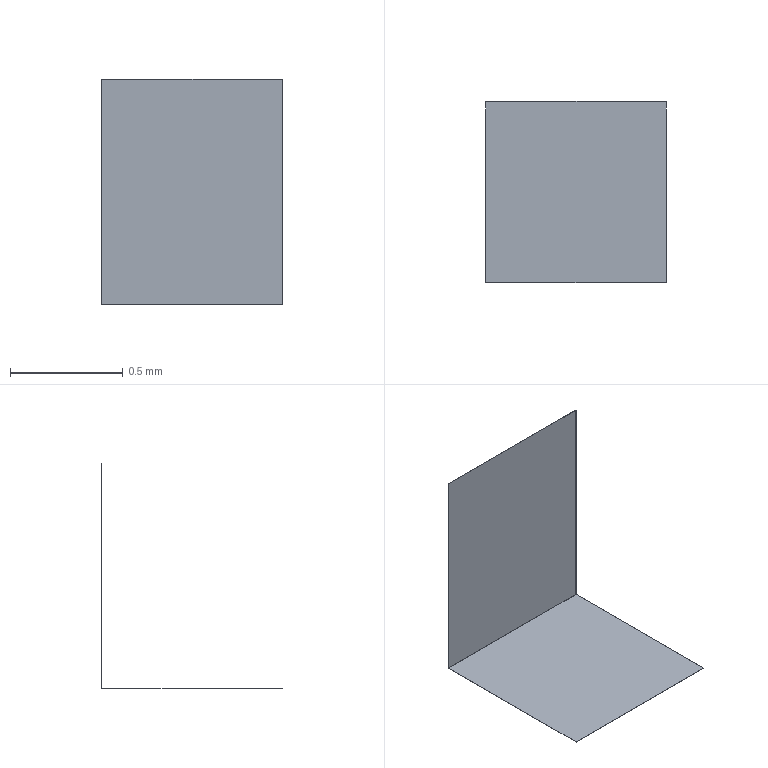Part | STEP file | RJ-USIO-V1_2-220411_9 | 1 solid | 14 faces | box 0.8 x 0.801 x 1 mm | volume 0.00144 mm3 | plane 14
STEP:
#1=CARTESIAN_POINT('',(0.,0.,0.));
#2=DIRECTION('',(0.,0.,1.));
#3=DIRECTION('',(1.,0.,0.));
#4=AXIS2_PLACEMENT_3D('',#1,#2,#3);
#5=CARTESIAN_POINT('',(24.9,60.501,1.));
#6=VERTEX_POINT('',#5);
#7=CARTESIAN_POINT('',(24.1,60.501,1.));
#8=VERTEX_POINT('',#7);
#9=CARTESIAN_POINT('',(24.9,60.501,1.));
#10=DIRECTION('',(-1.,-0.000000012,0.));
#11=VECTOR('',#10,1.);
#12=LINE('',#9,#11);
#13=CARTESIAN_POINT('',(24.1,60.501,0.));
#14=DIRECTION('',(0.000000012,-1.,0.));
#15=DIRECTION('',(0.,0.,1.));
#16=AXIS2_PLACEMENT_3D('',#13,#14,#15);
#17=PLANE('',#16);
#18=CARTESIAN_POINT('',(1.,-0.8));
#19=DIRECTION('',(0.,1.));
#20=VECTOR('',#19,1.);
#21=LINE('',#18,#20);
#22=(GEOMETRIC_REPRESENTATION_CONTEXT(2)PARAMETRIC_REPRESENTATION_CONTEXT()REPRESENTATION_CONTEXT('',''));
#23=DEFINITIONAL_REPRESENTATION('',(#21),#22);
#24=PCURVE('',#17,#23);
#25=CARTESIAN_POINT('',(24.1,60.5,1.));
#26=DIRECTION('',(0.,0.,-1.));
#27=DIRECTION('',(-1.,-0.000000012,0.));
#28=AXIS2_PLACEMENT_3D('',#25,#26,#27);
#29=PLANE('',#28);
#30=CARTESIAN_POINT('',(-0.8,0.001));
#31=DIRECTION('',(1.,0.));
#32=VECTOR('',#31,1.);
#33=LINE('',#30,#32);
#34=(GEOMETRIC_REPRESENTATION_CONTEXT(2)PARAMETRIC_REPRESENTATION_CONTEXT()REPRESENTATION_CONTEXT('',''));
#35=DEFINITIONAL_REPRESENTATION('',(#33),#34);
#36=PCURVE('',#29,#35);
#37=SURFACE_CURVE('',#12,(#24,#36),.PCURVE_S1.);
#38=EDGE_CURVE('',#6,#8,#37,.T.);
#39=ORIENTED_EDGE('',*,*,#38,.T.);
#40=CARTESIAN_POINT('',(24.1,60.501,0.001));
#41=VERTEX_POINT('',#40);
#42=CARTESIAN_POINT('',(24.1,60.501,1.));
#43=DIRECTION('',(0.,0.,-1.));
#44=VECTOR('',#43,1.);
#45=LINE('',#42,#44);
#46=CARTESIAN_POINT('',(1.,0.));
#47=DIRECTION('',(-1.,0.));
#48=VECTOR('',#47,1.);
#49=LINE('',#46,#48);
#50=(GEOMETRIC_REPRESENTATION_CONTEXT(2)PARAMETRIC_REPRESENTATION_CONTEXT()REPRESENTATION_CONTEXT('',''));
#51=DEFINITIONAL_REPRESENTATION('',(#49),#50);
#52=PCURVE('',#17,#51);
#53=CARTESIAN_POINT('',(24.1,60.5,0.));
#54=DIRECTION('',(1.,0.000000012,0.));
#55=DIRECTION('',(0.,0.,-1.));
#56=AXIS2_PLACEMENT_3D('',#53,#54,#55);
#57=PLANE('',#56);
#58=CARTESIAN_POINT('',(-1.,0.001));
#59=DIRECTION('',(1.,0.));
#60=VECTOR('',#59,1.);
#61=LINE('',#58,#60);
#62=(GEOMETRIC_REPRESENTATION_CONTEXT(2)PARAMETRIC_REPRESENTATION_CONTEXT()REPRESENTATION_CONTEXT('',''));
#63=DEFINITIONAL_REPRESENTATION('',(#61),#62);
#64=PCURVE('',#57,#63);
#65=SURFACE_CURVE('',#45,(#52,#64),.PCURVE_S1.);
#66=EDGE_CURVE('',#8,#41,#65,.T.);
#67=ORIENTED_EDGE('',*,*,#66,.T.);
#68=CARTESIAN_POINT('',(24.9,60.501,0.001));
#69=VERTEX_POINT('',#68);
#70=CARTESIAN_POINT('',(24.1,60.501,0.001));
#71=DIRECTION('',(1.,0.000000012,0.));
#72=VECTOR('',#71,1.);
#73=LINE('',#70,#72);
#74=CARTESIAN_POINT('',(0.001,0.));
#75=DIRECTION('',(0.,-1.));
#76=VECTOR('',#75,1.);
#77=LINE('',#74,#76);
#78=(GEOMETRIC_REPRESENTATION_CONTEXT(2)PARAMETRIC_REPRESENTATION_CONTEXT()REPRESENTATION_CONTEXT('',''));
#79=DEFINITIONAL_REPRESENTATION('',(#77),#78);
#80=PCURVE('',#17,#79);
#81=CARTESIAN_POINT('',(24.9,60.501,0.));
#82=DIRECTION('',(0.000000012,-1.,0.));
#83=DIRECTION('',(1.,0.000000012,0.));
#84=AXIS2_PLACEMENT_3D('',#81,#82,#83);
#85=PLANE('',#84);
#86=CARTESIAN_POINT('',(-0.8,0.001));
#87=DIRECTION('',(1.,0.));
#88=VECTOR('',#87,1.);
#89=LINE('',#86,#88);
#90=(GEOMETRIC_REPRESENTATION_CONTEXT(2)PARAMETRIC_REPRESENTATION_CONTEXT()REPRESENTATION_CONTEXT('',''));
#91=DEFINITIONAL_REPRESENTATION('',(#89),#90);
#92=PCURVE('',#85,#91);
#93=SURFACE_CURVE('',#73,(#80,#92),.PCURVE_S1.);
#94=EDGE_CURVE('',#41,#69,#93,.T.);
#95=ORIENTED_EDGE('',*,*,#94,.T.);
#96=CARTESIAN_POINT('',(24.9,60.501,0.001));
#97=DIRECTION('',(0.,0.,1.));
#98=VECTOR('',#97,1.);
#99=LINE('',#96,#98);
#100=CARTESIAN_POINT('',(0.001,-0.8));
#101=DIRECTION('',(1.,0.));
#102=VECTOR('',#101,1.);
#103=LINE('',#100,#102);
#104=(GEOMETRIC_REPRESENTATION_CONTEXT(2)PARAMETRIC_REPRESENTATION_CONTEXT()REPRESENTATION_CONTEXT('',''));
#105=DEFINITIONAL_REPRESENTATION('',(#103),#104);
#106=PCURVE('',#17,#105);
#107=CARTESIAN_POINT('',(24.9,60.5,1.));
#108=DIRECTION('',(-1.,-0.000000012,0.));
#109=DIRECTION('',(0.,0.,1.));
#110=AXIS2_PLACEMENT_3D('',#107,#108,#109);
#111=PLANE('',#110);
#112=CARTESIAN_POINT('',(-0.999,0.001));
#113=DIRECTION('',(1.,0.));
#114=VECTOR('',#113,1.);
#115=LINE('',#112,#114);
#116=(GEOMETRIC_REPRESENTATION_CONTEXT(2)PARAMETRIC_REPRESENTATION_CONTEXT()REPRESENTATION_CONTEXT('',''));
#117=DEFINITIONAL_REPRESENTATION('',(#115),#116);
#118=PCURVE('',#111,#117);
#119=SURFACE_CURVE('',#99,(#106,#118),.PCURVE_S1.);
#120=EDGE_CURVE('',#69,#6,#119,.T.);
#121=ORIENTED_EDGE('',*,*,#120,.T.);
#122=EDGE_LOOP('',(#39,#67,#95,#121));
#123=FACE_BOUND('',#122,.F.);
#124=ADVANCED_FACE('',(#123),#17,.F.);
#125=CARTESIAN_POINT('',(24.9,60.5,1.));
#126=VERTEX_POINT('',#125);
#127=CARTESIAN_POINT('',(24.1,60.5,1.));
#128=VERTEX_POINT('',#127);
#129=CARTESIAN_POINT('',(24.9,60.5,1.));
#130=DIRECTION('',(-1.,-0.000000012,0.));
#131=VECTOR('',#130,1.);
#132=LINE('',#129,#131);
#133=CARTESIAN_POINT('',(-0.8,0.));
#134=DIRECTION('',(1.,0.));
#135=VECTOR('',#134,1.);
#136=LINE('',#133,#135);
#137=(GEOMETRIC_REPRESENTATION_CONTEXT(2)PARAMETRIC_REPRESENTATION_CONTEXT()REPRESENTATION_CONTEXT('',''));
#138=DEFINITIONAL_REPRESENTATION('',(#136),#137);
#139=PCURVE('',#29,#138);
#140=CARTESIAN_POINT('',(24.1,60.5,0.));
#141=DIRECTION('',(0.000000012,-1.,0.));
#142=DIRECTION('',(0.,0.,1.));
#143=AXIS2_PLACEMENT_3D('',#140,#141,#142);
#144=PLANE('',#143);
#145=CARTESIAN_POINT('',(1.,-0.8));
#146=DIRECTION('',(0.,1.));
#147=VECTOR('',#146,1.);
#148=LINE('',#145,#147);
#149=(GEOMETRIC_REPRESENTATION_CONTEXT(2)PARAMETRIC_REPRESENTATION_CONTEXT()REPRESENTATION_CONTEXT('',''));
#150=DEFINITIONAL_REPRESENTATION('',(#148),#149);
#151=PCURVE('',#144,#150);
#152=SURFACE_CURVE('',#132,(#139,#151),.PCURVE_S1.);
#153=EDGE_CURVE('',#126,#128,#152,.T.);
#154=ORIENTED_EDGE('',*,*,#153,.T.);
#155=CARTESIAN_POINT('',(24.1,60.501,1.));
#156=DIRECTION('',(0.000000012,-1.,0.));
#157=VECTOR('',#156,1.);
#158=LINE('',#155,#157);
#159=CARTESIAN_POINT('',(0.,0.001));
#160=DIRECTION('',(0.,-1.));
#161=VECTOR('',#160,1.);
#162=LINE('',#159,#161);
#163=(GEOMETRIC_REPRESENTATION_CONTEXT(2)PARAMETRIC_REPRESENTATION_CONTEXT()REPRESENTATION_CONTEXT('',''));
#164=DEFINITIONAL_REPRESENTATION('',(#162),#163);
#165=PCURVE('',#29,#164);
#166=CARTESIAN_POINT('',(-1.,0.001));
#167=DIRECTION('',(0.,-1.));
#168=VECTOR('',#167,1.);
#169=LINE('',#166,#168);
#170=(GEOMETRIC_REPRESENTATION_CONTEXT(2)PARAMETRIC_REPRESENTATION_CONTEXT()REPRESENTATION_CONTEXT('',''));
#171=DEFINITIONAL_REPRESENTATION('',(#169),#170);
#172=PCURVE('',#57,#171);
#173=SURFACE_CURVE('',#158,(#165,#172),.PCURVE_S1.);
#174=EDGE_CURVE('',#8,#128,#173,.T.);
#175=ORIENTED_EDGE('',*,*,#174,.F.);
#176=ORIENTED_EDGE('',*,*,#38,.F.);
#177=CARTESIAN_POINT('',(24.9,60.501,1.));
#178=DIRECTION('',(0.000000012,-1.,0.));
#179=VECTOR('',#178,1.);
#180=LINE('',#177,#179);
#181=CARTESIAN_POINT('',(-0.8,0.001));
#182=DIRECTION('',(0.,-1.));
#183=VECTOR('',#182,1.);
#184=LINE('',#181,#183);
#185=(GEOMETRIC_REPRESENTATION_CONTEXT(2)PARAMETRIC_REPRESENTATION_CONTEXT()REPRESENTATION_CONTEXT('',''));
#186=DEFINITIONAL_REPRESENTATION('',(#184),#185);
#187=PCURVE('',#29,#186);
#188=CARTESIAN_POINT('',(0.,0.001));
#189=DIRECTION('',(0.,-1.));
#190=VECTOR('',#189,1.);
#191=LINE('',#188,#190);
#192=(GEOMETRIC_REPRESENTATION_CONTEXT(2)PARAMETRIC_REPRESENTATION_CONTEXT()REPRESENTATION_CONTEXT('',''));
#193=DEFINITIONAL_REPRESENTATION('',(#191),#192);
#194=PCURVE('',#111,#193);
#195=SURFACE_CURVE('',#180,(#187,#194),.PCURVE_S1.);
#196=EDGE_CURVE('',#6,#126,#195,.T.);
#197=ORIENTED_EDGE('',*,*,#196,.T.);
#198=EDGE_LOOP('',(#154,#175,#176,#197));
#199=FACE_BOUND('',#198,.F.);
#200=ADVANCED_FACE('',(#199),#29,.F.);
#201=CARTESIAN_POINT('',(24.1,60.5,0.001));
#202=VERTEX_POINT('',#201);
#203=CARTESIAN_POINT('',(24.1,60.5,1.));
#204=DIRECTION('',(0.,0.,-1.));
#205=VECTOR('',#204,1.);
#206=LINE('',#203,#205);
#207=CARTESIAN_POINT('',(1.,0.));
#208=DIRECTION('',(-1.,0.));
#209=VECTOR('',#208,1.);
#210=LINE('',#207,#209);
#211=(GEOMETRIC_REPRESENTATION_CONTEXT(2)PARAMETRIC_REPRESENTATION_CONTEXT()REPRESENTATION_CONTEXT('',''));
#212=DEFINITIONAL_REPRESENTATION('',(#210),#211);
#213=PCURVE('',#144,#212);
#214=CARTESIAN_POINT('',(-1.,0.));
#215=DIRECTION('',(1.,0.));
#216=VECTOR('',#215,1.);
#217=LINE('',#214,#216);
#218=(GEOMETRIC_REPRESENTATION_CONTEXT(2)PARAMETRIC_REPRESENTATION_CONTEXT()REPRESENTATION_CONTEXT('',''));
#219=DEFINITIONAL_REPRESENTATION('',(#217),#218);
#220=PCURVE('',#57,#219);
#221=SURFACE_CURVE('',#206,(#213,#220),.PCURVE_S1.);
#222=EDGE_CURVE('',#128,#202,#221,.T.);
#223=ORIENTED_EDGE('',*,*,#222,.F.);
#224=ORIENTED_EDGE('',*,*,#153,.F.);
#225=CARTESIAN_POINT('',(24.9,60.5,0.001));
#226=VERTEX_POINT('',#225);
#227=CARTESIAN_POINT('',(24.9,60.5,0.001));
#228=DIRECTION('',(0.,0.,1.));
#229=VECTOR('',#228,1.);
#230=LINE('',#227,#229);
#231=CARTESIAN_POINT('',(0.001,-0.8));
#232=DIRECTION('',(1.,0.));
#233=VECTOR('',#232,1.);
#234=LINE('',#231,#233);
#235=(GEOMETRIC_REPRESENTATION_CONTEXT(2)PARAMETRIC_REPRESENTATION_CONTEXT()REPRESENTATION_CONTEXT('',''));
#236=DEFINITIONAL_REPRESENTATION('',(#234),#235);
#237=PCURVE('',#144,#236);
#238=CARTESIAN_POINT('',(-0.999,0.));
#239=DIRECTION('',(1.,0.));
#240=VECTOR('',#239,1.);
#241=LINE('',#238,#240);
#242=(GEOMETRIC_REPRESENTATION_CONTEXT(2)PARAMETRIC_REPRESENTATION_CONTEXT()REPRESENTATION_CONTEXT('',''));
#243=DEFINITIONAL_REPRESENTATION('',(#241),#242);
#244=PCURVE('',#111,#243);
#245=SURFACE_CURVE('',#230,(#237,#244),.PCURVE_S1.);
#246=EDGE_CURVE('',#226,#126,#245,.T.);
#247=ORIENTED_EDGE('',*,*,#246,.F.);
#248=CARTESIAN_POINT('',(24.1,60.5,0.001));
#249=DIRECTION('',(1.,0.000000012,0.));
#250=VECTOR('',#249,1.);
#251=LINE('',#248,#250);
#252=CARTESIAN_POINT('',(0.001,0.));
#253=DIRECTION('',(0.,-1.));
#254=VECTOR('',#253,1.);
#255=LINE('',#252,#254);
#256=(GEOMETRIC_REPRESENTATION_CONTEXT(2)PARAMETRIC_REPRESENTATION_CONTEXT()REPRESENTATION_CONTEXT('',''));
#257=DEFINITIONAL_REPRESENTATION('',(#255),#256);
#258=PCURVE('',#144,#257);
#259=CARTESIAN_POINT('',(24.1,60.501,0.001));
#260=DIRECTION('',(0.,0.,-1.));
#261=DIRECTION('',(0.000000012,-1.,0.));
#262=AXIS2_PLACEMENT_3D('',#259,#260,#261);
#263=PLANE('',#262);
#264=CARTESIAN_POINT('',(0.001,0.));
#265=DIRECTION('',(0.,-1.));
#266=VECTOR('',#265,1.);
#267=LINE('',#264,#266);
#268=(GEOMETRIC_REPRESENTATION_CONTEXT(2)PARAMETRIC_REPRESENTATION_CONTEXT()REPRESENTATION_CONTEXT('',''));
#269=DEFINITIONAL_REPRESENTATION('',(#267),#268);
#270=PCURVE('',#263,#269);
#271=SURFACE_CURVE('',#251,(#258,#270),.PCURVE_S1.);
#272=EDGE_CURVE('',#202,#226,#271,.T.);
#273=ORIENTED_EDGE('',*,*,#272,.F.);
#274=EDGE_LOOP('',(#223,#224,#247,#273));
#275=FACE_BOUND('',#274,.F.);
#276=ADVANCED_FACE('',(#275),#144,.T.);
#277=ORIENTED_EDGE('',*,*,#174,.T.);
#278=ORIENTED_EDGE('',*,*,#222,.T.);
#279=CARTESIAN_POINT('',(24.1,60.5,0.001));
#280=DIRECTION('',(-0.000000012,1.,0.));
#281=VECTOR('',#280,1.);
#282=LINE('',#279,#281);
#283=CARTESIAN_POINT('',(-0.001,0.));
#284=DIRECTION('',(0.,1.));
#285=VECTOR('',#284,1.);
#286=LINE('',#283,#285);
#287=(GEOMETRIC_REPRESENTATION_CONTEXT(2)PARAMETRIC_REPRESENTATION_CONTEXT()REPRESENTATION_CONTEXT('',''));
#288=DEFINITIONAL_REPRESENTATION('',(#286),#287);
#289=PCURVE('',#57,#288);
#290=CARTESIAN_POINT('',(24.1,60.5,0.));
#291=DIRECTION('',(1.,0.000000012,0.));
#292=DIRECTION('',(0.,0.,-1.));
#293=AXIS2_PLACEMENT_3D('',#290,#291,#292);
#294=PLANE('',#293);
#295=CARTESIAN_POINT('',(-0.001,0.));
#296=DIRECTION('',(0.,1.));
#297=VECTOR('',#296,1.);
#298=LINE('',#295,#297);
#299=(GEOMETRIC_REPRESENTATION_CONTEXT(2)PARAMETRIC_REPRESENTATION_CONTEXT()REPRESENTATION_CONTEXT('',''));
#300=DEFINITIONAL_REPRESENTATION('',(#298),#299);
#301=PCURVE('',#294,#300);
#302=SURFACE_CURVE('',#282,(#289,#301),.PCURVE_S1.);
#303=EDGE_CURVE('',#202,#41,#302,.T.);
#304=ORIENTED_EDGE('',*,*,#303,.T.);
#305=ORIENTED_EDGE('',*,*,#66,.F.);
#306=EDGE_LOOP('',(#277,#278,#304,#305));
#307=FACE_BOUND('',#306,.F.);
#308=ADVANCED_FACE('',(#307),#57,.F.);
#309=ORIENTED_EDGE('',*,*,#303,.F.);
#310=CARTESIAN_POINT('',(24.1,60.5,0.));
#311=VERTEX_POINT('',#310);
#312=CARTESIAN_POINT('',(24.1,60.5,0.001));
#313=DIRECTION('',(0.,0.,-1.));
#314=VECTOR('',#313,1.);
#315=LINE('',#312,#314);
#316=CARTESIAN_POINT('',(-0.001,0.));
#317=DIRECTION('',(1.,0.));
#318=VECTOR('',#317,1.);
#319=LINE('',#316,#318);
#320=(GEOMETRIC_REPRESENTATION_CONTEXT(2)PARAMETRIC_REPRESENTATION_CONTEXT()REPRESENTATION_CONTEXT('',''));
#321=DEFINITIONAL_REPRESENTATION('',(#319),#320);
#322=PCURVE('',#294,#321);
#323=CARTESIAN_POINT('',(24.1,60.501,0.));
#324=DIRECTION('',(1.,0.000000012,0.));
#325=DIRECTION('',(-0.000000012,1.,0.));
#326=AXIS2_PLACEMENT_3D('',#323,#324,#325);
#327=PLANE('',#326);
#328=CARTESIAN_POINT('',(-0.001,0.001));
#329=DIRECTION('',(0.,-1.));
#330=VECTOR('',#329,1.);
#331=LINE('',#328,#330);
#332=(GEOMETRIC_REPRESENTATION_CONTEXT(2)PARAMETRIC_REPRESENTATION_CONTEXT()REPRESENTATION_CONTEXT('',''));
#333=DEFINITIONAL_REPRESENTATION('',(#331),#332);
#334=PCURVE('',#327,#333);
#335=SURFACE_CURVE('',#315,(#322,#334),.PCURVE_S1.);
#336=EDGE_CURVE('',#202,#311,#335,.T.);
#337=ORIENTED_EDGE('',*,*,#336,.T.);
#338=CARTESIAN_POINT('',(24.1,60.501,0.));
#339=VERTEX_POINT('',#338);
#340=CARTESIAN_POINT('',(24.1,60.501,0.));
#341=DIRECTION('',(0.000000012,-1.,0.));
#342=VECTOR('',#341,1.);
#343=LINE('',#340,#342);
#344=CARTESIAN_POINT('',(0.,0.001));
#345=DIRECTION('',(0.,-1.));
#346=VECTOR('',#345,1.);
#347=LINE('',#344,#346);
#348=(GEOMETRIC_REPRESENTATION_CONTEXT(2)PARAMETRIC_REPRESENTATION_CONTEXT()REPRESENTATION_CONTEXT('',''));
#349=DEFINITIONAL_REPRESENTATION('',(#347),#348);
#350=PCURVE('',#294,#349);
#351=CARTESIAN_POINT('',(24.1,60.501,0.));
#352=DIRECTION('',(0.,0.,-1.));
#353=DIRECTION('',(0.000000012,-1.,0.));
#354=AXIS2_PLACEMENT_3D('',#351,#352,#353);
#355=PLANE('',#354);
#356=CARTESIAN_POINT('',(0.,0.));
#357=DIRECTION('',(1.,0.));
#358=VECTOR('',#357,1.);
#359=LINE('',#356,#358);
#360=(GEOMETRIC_REPRESENTATION_CONTEXT(2)PARAMETRIC_REPRESENTATION_CONTEXT()REPRESENTATION_CONTEXT('',''));
#361=DEFINITIONAL_REPRESENTATION('',(#359),#360);
#362=PCURVE('',#355,#361);
#363=SURFACE_CURVE('',#343,(#350,#362),.PCURVE_S1.);
#364=EDGE_CURVE('',#339,#311,#363,.T.);
#365=ORIENTED_EDGE('',*,*,#364,.F.);
#366=CARTESIAN_POINT('',(24.1,60.501,0.001));
#367=DIRECTION('',(0.,0.,-1.));
#368=VECTOR('',#367,1.);
#369=LINE('',#366,#368);
#370=CARTESIAN_POINT('',(-0.001,0.001));
#371=DIRECTION('',(1.,0.));
#372=VECTOR('',#371,1.);
#373=LINE('',#370,#372);
#374=(GEOMETRIC_REPRESENTATION_CONTEXT(2)PARAMETRIC_REPRESENTATION_CONTEXT()REPRESENTATION_CONTEXT('',''));
#375=DEFINITIONAL_REPRESENTATION('',(#373),#374);
#376=PCURVE('',#294,#375);
#377=CARTESIAN_POINT('',(-0.8,0.001));
#378=DIRECTION('',(0.,-1.));
#379=VECTOR('',#378,1.);
#380=LINE('',#377,#379);
#381=(GEOMETRIC_REPRESENTATION_CONTEXT(2)PARAMETRIC_REPRESENTATION_CONTEXT()REPRESENTATION_CONTEXT('',''));
#382=DEFINITIONAL_REPRESENTATION('',(#380),#381);
#383=PCURVE('',#85,#382);
#384=SURFACE_CURVE('',#369,(#376,#383),.PCURVE_S1.);
#385=EDGE_CURVE('',#41,#339,#384,.T.);
#386=ORIENTED_EDGE('',*,*,#385,.F.);
#387=EDGE_LOOP('',(#309,#337,#365,#386));
#388=FACE_BOUND('',#387,.F.);
#389=ADVANCED_FACE('',(#388),#294,.F.);
#390=CARTESIAN_POINT('',(24.1,59.7,0.001));
#391=VERTEX_POINT('',#390);
#392=CARTESIAN_POINT('',(24.1,59.7,0.));
#393=VERTEX_POINT('',#392);
#394=CARTESIAN_POINT('',(24.1,59.7,0.001));
#395=DIRECTION('',(0.,0.,-1.));
#396=VECTOR('',#395,1.);
#397=LINE('',#394,#396);
#398=CARTESIAN_POINT('',(-0.801,0.001));
#399=DIRECTION('',(0.,-1.));
#400=VECTOR('',#399,1.);
#401=LINE('',#398,#400);
#402=(GEOMETRIC_REPRESENTATION_CONTEXT(2)PARAMETRIC_REPRESENTATION_CONTEXT()REPRESENTATION_CONTEXT('',''));
#403=DEFINITIONAL_REPRESENTATION('',(#401),#402);
#404=PCURVE('',#327,#403);
#405=CARTESIAN_POINT('',(24.1,59.7,0.));
#406=DIRECTION('',(-0.000000012,1.,0.));
#407=DIRECTION('',(-1.,-0.000000012,0.));
#408=AXIS2_PLACEMENT_3D('',#405,#406,#407);
#409=PLANE('',#408);
#410=CARTESIAN_POINT('',(0.,0.001));
#411=DIRECTION('',(0.,-1.));
#412=VECTOR('',#411,1.);
#413=LINE('',#410,#412);
#414=(GEOMETRIC_REPRESENTATION_CONTEXT(2)PARAMETRIC_REPRESENTATION_CONTEXT()REPRESENTATION_CONTEXT('',''));
#415=DEFINITIONAL_REPRESENTATION('',(#413),#414);
#416=PCURVE('',#409,#415);
#417=SURFACE_CURVE('',#397,(#404,#416),.PCURVE_S1.);
#418=EDGE_CURVE('',#391,#393,#417,.T.);
#419=ORIENTED_EDGE('',*,*,#418,.T.);
#420=CARTESIAN_POINT('',(24.1,59.7,0.));
#421=DIRECTION('',(-0.000000012,1.,0.));
#422=VECTOR('',#421,1.);
#423=LINE('',#420,#422);
#424=CARTESIAN_POINT('',(-0.801,0.));
#425=DIRECTION('',(1.,0.));
#426=VECTOR('',#425,1.);
#427=LINE('',#424,#426);
#428=(GEOMETRIC_REPRESENTATION_CONTEXT(2)PARAMETRIC_REPRESENTATION_CONTEXT()REPRESENTATION_CONTEXT('',''));
#429=DEFINITIONAL_REPRESENTATION('',(#427),#428);
#430=PCURVE('',#327,#429);
#431=CARTESIAN_POINT('',(24.1,60.501,0.));
#432=DIRECTION('',(0.,0.,-1.));
#433=DIRECTION('',(0.000000012,-1.,0.));
#434=AXIS2_PLACEMENT_3D('',#431,#432,#433);
#435=PLANE('',#434);
#436=CARTESIAN_POINT('',(0.801,0.));
#437=DIRECTION('',(-1.,0.));
#438=VECTOR('',#437,1.);
#439=LINE('',#436,#438);
#440=(GEOMETRIC_REPRESENTATION_CONTEXT(2)PARAMETRIC_REPRESENTATION_CONTEXT()REPRESENTATION_CONTEXT('',''));
#441=DEFINITIONAL_REPRESENTATION('',(#439),#440);
#442=PCURVE('',#435,#441);
#443=SURFACE_CURVE('',#423,(#430,#442),.PCURVE_S1.);
#444=EDGE_CURVE('',#393,#311,#443,.T.);
#445=ORIENTED_EDGE('',*,*,#444,.T.);
#446=ORIENTED_EDGE('',*,*,#336,.F.);
#447=CARTESIAN_POINT('',(24.1,59.7,0.001));
#448=DIRECTION('',(-0.000000012,1.,0.));
#449=VECTOR('',#448,1.);
#450=LINE('',#447,#449);
#451=CARTESIAN_POINT('',(-0.801,0.001));
#452=DIRECTION('',(1.,0.));
#453=VECTOR('',#452,1.);
#454=LINE('',#451,#453);
#455=(GEOMETRIC_REPRESENTATION_CONTEXT(2)PARAMETRIC_REPRESENTATION_CONTEXT()REPRESENTATION_CONTEXT('',''));
#456=DEFINITIONAL_REPRESENTATION('',(#454),#455);
#457=PCURVE('',#327,#456);
#458=CARTESIAN_POINT('',(0.801,0.));
#459=DIRECTION('',(-1.,0.));
#460=VECTOR('',#459,1.);
#461=LINE('',#458,#460);
#462=(GEOMETRIC_REPRESENTATION_CONTEXT(2)PARAMETRIC_REPRESENTATION_CONTEXT()REPRESENTATION_CONTEXT('',''));
#463=DEFINITIONAL_REPRESENTATION('',(#461),#462);
#464=PCURVE('',#263,#463);
#465=SURFACE_CURVE('',#450,(#457,#464),.PCURVE_S1.);
#466=EDGE_CURVE('',#391,#202,#465,.T.);
#467=ORIENTED_EDGE('',*,*,#466,.F.);
#468=EDGE_LOOP('',(#419,#445,#446,#467));
#469=FACE_BOUND('',#468,.F.);
#470=ADVANCED_FACE('',(#469),#327,.F.);
#471=CARTESIAN_POINT('',(24.9,59.7,0.));
#472=VERTEX_POINT('',#471);
#473=CARTESIAN_POINT('',(24.9,59.7,0.));
#474=DIRECTION('',(-1.,-0.000000012,0.));
#475=VECTOR('',#474,1.);
#476=LINE('',#473,#475);
#477=CARTESIAN_POINT('',(-0.8,0.));
#478=DIRECTION('',(1.,0.));
#479=VECTOR('',#478,1.);
#480=LINE('',#477,#479);
#481=(GEOMETRIC_REPRESENTATION_CONTEXT(2)PARAMETRIC_REPRESENTATION_CONTEXT()REPRESENTATION_CONTEXT('',''));
#482=DEFINITIONAL_REPRESENTATION('',(#480),#481);
#483=PCURVE('',#409,#482);
#484=CARTESIAN_POINT('',(0.801,-0.8));
#485=DIRECTION('',(0.,1.));
#486=VECTOR('',#485,1.);
#487=LINE('',#484,#486);
#488=(GEOMETRIC_REPRESENTATION_CONTEXT(2)PARAMETRIC_REPRESENTATION_CONTEXT()REPRESENTATION_CONTEXT('',''));
#489=DEFINITIONAL_REPRESENTATION('',(#487),#488);
#490=PCURVE('',#435,#489);
#491=SURFACE_CURVE('',#476,(#483,#490),.PCURVE_S1.);
#492=EDGE_CURVE('',#472,#393,#491,.T.);
#493=ORIENTED_EDGE('',*,*,#492,.T.);
#494=ORIENTED_EDGE('',*,*,#418,.F.);
#495=CARTESIAN_POINT('',(24.9,59.7,0.001));
#496=VERTEX_POINT('',#495);
#497=CARTESIAN_POINT('',(24.9,59.7,0.001));
#498=DIRECTION('',(-1.,-0.000000012,0.));
#499=VECTOR('',#498,1.);
#500=LINE('',#497,#499);
#501=CARTESIAN_POINT('',(-0.8,0.001));
#502=DIRECTION('',(1.,0.));
#503=VECTOR('',#502,1.);
#504=LINE('',#501,#503);
#505=(GEOMETRIC_REPRESENTATION_CONTEXT(2)PARAMETRIC_REPRESENTATION_CONTEXT()REPRESENTATION_CONTEXT('',''));
#506=DEFINITIONAL_REPRESENTATION('',(#504),#505);
#507=PCURVE('',#409,#506);
#508=CARTESIAN_POINT('',(0.801,-0.8));
#509=DIRECTION('',(0.,1.));
#510=VECTOR('',#509,1.);
#511=LINE('',#508,#510);
#512=(GEOMETRIC_REPRESENTATION_CONTEXT(2)PARAMETRIC_REPRESENTATION_CONTEXT()REPRESENTATION_CONTEXT('',''));
#513=DEFINITIONAL_REPRESENTATION('',(#511),#512);
#514=PCURVE('',#263,#513);
#515=SURFACE_CURVE('',#500,(#507,#514),.PCURVE_S1.);
#516=EDGE_CURVE('',#496,#391,#515,.T.);
#517=ORIENTED_EDGE('',*,*,#516,.F.);
#518=CARTESIAN_POINT('',(24.9,59.7,0.001));
#519=DIRECTION('',(0.,0.,-1.));
#520=VECTOR('',#519,1.);
#521=LINE('',#518,#520);
#522=CARTESIAN_POINT('',(-0.8,0.001));
#523=DIRECTION('',(0.,-1.));
#524=VECTOR('',#523,1.);
#525=LINE('',#522,#524);
#526=(GEOMETRIC_REPRESENTATION_CONTEXT(2)PARAMETRIC_REPRESENTATION_CONTEXT()REPRESENTATION_CONTEXT('',''));
#527=DEFINITIONAL_REPRESENTATION('',(#525),#526);
#528=PCURVE('',#409,#527);
#529=CARTESIAN_POINT('',(24.9,59.7,0.));
#530=DIRECTION('',(-1.,-0.000000012,0.));
#531=DIRECTION('',(0.000000012,-1.,0.));
#532=AXIS2_PLACEMENT_3D('',#529,#530,#531);
#533=PLANE('',#532);
#534=CARTESIAN_POINT('',(0.,0.001));
#535=DIRECTION('',(0.,-1.));
#536=VECTOR('',#535,1.);
#537=LINE('',#534,#536);
#538=(GEOMETRIC_REPRESENTATION_CONTEXT(2)PARAMETRIC_REPRESENTATION_CONTEXT()REPRESENTATION_CONTEXT('',''));
#539=DEFINITIONAL_REPRESENTATION('',(#537),#538);
#540=PCURVE('',#533,#539);
#541=SURFACE_CURVE('',#521,(#528,#540),.PCURVE_S1.);
#542=EDGE_CURVE('',#496,#472,#541,.T.);
#543=ORIENTED_EDGE('',*,*,#542,.T.);
#544=EDGE_LOOP('',(#493,#494,#517,#543));
#545=FACE_BOUND('',#544,.F.);
#546=ADVANCED_FACE('',(#545),#409,.F.);
#547=ORIENTED_EDGE('',*,*,#444,.F.);
#548=ORIENTED_EDGE('',*,*,#492,.F.);
#549=CARTESIAN_POINT('',(24.9,60.5,0.));
#550=VERTEX_POINT('',#549);
#551=CARTESIAN_POINT('',(24.9,60.5,0.));
#552=DIRECTION('',(0.000000012,-1.,0.));
#553=VECTOR('',#552,1.);
#554=LINE('',#551,#553);
#555=CARTESIAN_POINT('',(0.001,-0.8));
#556=DIRECTION('',(1.,0.));
#557=VECTOR('',#556,1.);
#558=LINE('',#555,#557);
#559=(GEOMETRIC_REPRESENTATION_CONTEXT(2)PARAMETRIC_REPRESENTATION_CONTEXT()REPRESENTATION_CONTEXT('',''));
#560=DEFINITIONAL_REPRESENTATION('',(#558),#559);
#561=PCURVE('',#435,#560);
#562=CARTESIAN_POINT('',(-0.8,0.));
#563=DIRECTION('',(1.,0.));
#564=VECTOR('',#563,1.);
#565=LINE('',#562,#564);
#566=(GEOMETRIC_REPRESENTATION_CONTEXT(2)PARAMETRIC_REPRESENTATION_CONTEXT()REPRESENTATION_CONTEXT('',''));
#567=DEFINITIONAL_REPRESENTATION('',(#565),#566);
#568=PCURVE('',#533,#567);
#569=SURFACE_CURVE('',#554,(#561,#568),.PCURVE_S1.);
#570=EDGE_CURVE('',#550,#472,#569,.T.);
#571=ORIENTED_EDGE('',*,*,#570,.F.);
#572=CARTESIAN_POINT('',(24.1,60.5,0.));
#573=DIRECTION('',(1.,0.000000012,0.));
#574=VECTOR('',#573,1.);
#575=LINE('',#572,#574);
#576=CARTESIAN_POINT('',(0.001,0.));
#577=DIRECTION('',(0.,-1.));
#578=VECTOR('',#577,1.);
#579=LINE('',#576,#578);
#580=(GEOMETRIC_REPRESENTATION_CONTEXT(2)PARAMETRIC_REPRESENTATION_CONTEXT()REPRESENTATION_CONTEXT('',''));
#581=DEFINITIONAL_REPRESENTATION('',(#579),#580);
#582=PCURVE('',#435,#581);
#583=CARTESIAN_POINT('',(0.001,0.));
#584=DIRECTION('',(0.,-1.));
#585=VECTOR('',#584,1.);
#586=LINE('',#583,#585);
#587=(GEOMETRIC_REPRESENTATION_CONTEXT(2)PARAMETRIC_REPRESENTATION_CONTEXT()REPRESENTATION_CONTEXT('',''));
#588=DEFINITIONAL_REPRESENTATION('',(#586),#587);
#589=PCURVE('',#355,#588);
#590=SURFACE_CURVE('',#575,(#582,#589),.PCURVE_S1.);
#591=EDGE_CURVE('',#311,#550,#590,.T.);
#592=ORIENTED_EDGE('',*,*,#591,.F.);
#593=EDGE_LOOP('',(#547,#548,#571,#592));
#594=FACE_BOUND('',#593,.F.);
#595=ADVANCED_FACE('',(#594),#435,.T.);
#596=CARTESIAN_POINT('',(24.9,60.5,0.));
#597=DIRECTION('',(0.,0.,1.));
#598=VECTOR('',#597,1.);
#599=LINE('',#596,#598);
#600=CARTESIAN_POINT('',(-0.8,0.));
#601=DIRECTION('',(0.,1.));
#602=VECTOR('',#601,1.);
#603=LINE('',#600,#602);
#604=(GEOMETRIC_REPRESENTATION_CONTEXT(2)PARAMETRIC_REPRESENTATION_CONTEXT()REPRESENTATION_CONTEXT('',''));
#605=DEFINITIONAL_REPRESENTATION('',(#603),#604);
#606=PCURVE('',#533,#605);
#607=CARTESIAN_POINT('',(24.9,60.5,1.));
#608=DIRECTION('',(-1.,-0.000000012,0.));
#609=DIRECTION('',(0.,0.,1.));
#610=AXIS2_PLACEMENT_3D('',#607,#608,#609);
#611=PLANE('',#610);
#612=CARTESIAN_POINT('',(-1.,0.));
#613=DIRECTION('',(1.,0.));
#614=VECTOR('',#613,1.);
#615=LINE('',#612,#614);
#616=(GEOMETRIC_REPRESENTATION_CONTEXT(2)PARAMETRIC_REPRESENTATION_CONTEXT()REPRESENTATION_CONTEXT('',''));
#617=DEFINITIONAL_REPRESENTATION('',(#615),#616);
#618=PCURVE('',#611,#617);
#619=SURFACE_CURVE('',#599,(#606,#618),.PCURVE_S1.);
#620=EDGE_CURVE('',#550,#226,#619,.T.);
#621=ORIENTED_EDGE('',*,*,#620,.F.);
#622=ORIENTED_EDGE('',*,*,#570,.T.);
#623=ORIENTED_EDGE('',*,*,#542,.F.);
#624=CARTESIAN_POINT('',(24.9,60.5,0.001));
#625=DIRECTION('',(0.000000012,-1.,0.));
#626=VECTOR('',#625,1.);
#627=LINE('',#624,#626);
#628=CARTESIAN_POINT('',(-0.8,0.001));
#629=DIRECTION('',(1.,0.));
#630=VECTOR('',#629,1.);
#631=LINE('',#628,#630);
#632=(GEOMETRIC_REPRESENTATION_CONTEXT(2)PARAMETRIC_REPRESENTATION_CONTEXT()REPRESENTATION_CONTEXT('',''));
#633=DEFINITIONAL_REPRESENTATION('',(#631),#632);
#634=PCURVE('',#533,#633);
#635=CARTESIAN_POINT('',(0.001,-0.8));
#636=DIRECTION('',(1.,0.));
#637=VECTOR('',#636,1.);
#638=LINE('',#635,#637);
#639=(GEOMETRIC_REPRESENTATION_CONTEXT(2)PARAMETRIC_REPRESENTATION_CONTEXT()REPRESENTATION_CONTEXT('',''));
#640=DEFINITIONAL_REPRESENTATION('',(#638),#639);
#641=PCURVE('',#263,#640);
#642=SURFACE_CURVE('',#627,(#634,#641),.PCURVE_S1.);
#643=EDGE_CURVE('',#226,#496,#642,.T.);
#644=ORIENTED_EDGE('',*,*,#643,.F.);
#645=EDGE_LOOP('',(#621,#622,#623,#644));
#646=FACE_BOUND('',#645,.F.);
#647=ADVANCED_FACE('',(#646),#533,.F.);
#648=CARTESIAN_POINT('',(24.9,60.501,0.));
#649=VERTEX_POINT('',#648);
#650=CARTESIAN_POINT('',(24.9,60.501,0.));
#651=DIRECTION('',(0.000000012,-1.,0.));
#652=VECTOR('',#651,1.);
#653=LINE('',#650,#652);
#654=CARTESIAN_POINT('',(-1.,0.001));
#655=DIRECTION('',(0.,-1.));
#656=VECTOR('',#655,1.);
#657=LINE('',#654,#656);
#658=(GEOMETRIC_REPRESENTATION_CONTEXT(2)PARAMETRIC_REPRESENTATION_CONTEXT()REPRESENTATION_CONTEXT('',''));
#659=DEFINITIONAL_REPRESENTATION('',(#657),#658);
#660=PCURVE('',#611,#659);
#661=CARTESIAN_POINT('',(0.,-0.8));
#662=DIRECTION('',(1.,0.));
#663=VECTOR('',#662,1.);
#664=LINE('',#661,#663);
#665=(GEOMETRIC_REPRESENTATION_CONTEXT(2)PARAMETRIC_REPRESENTATION_CONTEXT()REPRESENTATION_CONTEXT('',''));
#666=DEFINITIONAL_REPRESENTATION('',(#664),#665);
#667=PCURVE('',#355,#666);
#668=SURFACE_CURVE('',#653,(#660,#667),.PCURVE_S1.);
#669=EDGE_CURVE('',#649,#550,#668,.T.);
#670=ORIENTED_EDGE('',*,*,#669,.T.);
#671=ORIENTED_EDGE('',*,*,#620,.T.);
#672=CARTESIAN_POINT('',(24.9,60.501,0.001));
#673=DIRECTION('',(0.000000012,-1.,0.));
#674=VECTOR('',#673,1.);
#675=LINE('',#672,#674);
#676=CARTESIAN_POINT('',(-0.999,0.001));
#677=DIRECTION('',(0.,-1.));
#678=VECTOR('',#677,1.);
#679=LINE('',#676,#678);
#680=(GEOMETRIC_REPRESENTATION_CONTEXT(2)PARAMETRIC_REPRESENTATION_CONTEXT()REPRESENTATION_CONTEXT('',''));
#681=DEFINITIONAL_REPRESENTATION('',(#679),#680);
#682=PCURVE('',#611,#681);
#683=CARTESIAN_POINT('',(-0.999,0.001));
#684=DIRECTION('',(0.,-1.));
#685=VECTOR('',#684,1.);
#686=LINE('',#683,#685);
#687=(GEOMETRIC_REPRESENTATION_CONTEXT(2)PARAMETRIC_REPRESENTATION_CONTEXT()REPRESENTATION_CONTEXT('',''));
#688=DEFINITIONAL_REPRESENTATION('',(#686),#687);
#689=PCURVE('',#111,#688);
#690=SURFACE_CURVE('',#675,(#682,#689),.PCURVE_S1.);
#691=EDGE_CURVE('',#69,#226,#690,.T.);
#692=ORIENTED_EDGE('',*,*,#691,.F.);
#693=CARTESIAN_POINT('',(24.9,60.501,0.001));
#694=DIRECTION('',(0.,0.,-1.));
#695=VECTOR('',#694,1.);
#696=LINE('',#693,#695);
#697=CARTESIAN_POINT('',(-0.999,0.001));
#698=DIRECTION('',(-1.,0.));
#699=VECTOR('',#698,1.);
#700=LINE('',#697,#699);
#701=(GEOMETRIC_REPRESENTATION_CONTEXT(2)PARAMETRIC_REPRESENTATION_CONTEXT()REPRESENTATION_CONTEXT('',''));
#702=DEFINITIONAL_REPRESENTATION('',(#700),#701);
#703=PCURVE('',#611,#702);
#704=CARTESIAN_POINT('',(0.,0.001));
#705=DIRECTION('',(0.,-1.));
#706=VECTOR('',#705,1.);
#707=LINE('',#704,#706);
#708=(GEOMETRIC_REPRESENTATION_CONTEXT(2)PARAMETRIC_REPRESENTATION_CONTEXT()REPRESENTATION_CONTEXT('',''));
#709=DEFINITIONAL_REPRESENTATION('',(#707),#708);
#710=PCURVE('',#85,#709);
#711=SURFACE_CURVE('',#696,(#703,#710),.PCURVE_S1.);
#712=EDGE_CURVE('',#69,#649,#711,.T.);
#713=ORIENTED_EDGE('',*,*,#712,.T.);
#714=EDGE_LOOP('',(#670,#671,#692,#713));
#715=FACE_BOUND('',#714,.F.);
#716=ADVANCED_FACE('',(#715),#611,.F.);
#717=ORIENTED_EDGE('',*,*,#591,.T.);
#718=ORIENTED_EDGE('',*,*,#669,.F.);
#719=CARTESIAN_POINT('',(24.1,60.501,0.));
#720=DIRECTION('',(1.,0.000000012,0.));
#721=VECTOR('',#720,1.);
#722=LINE('',#719,#721);
#723=CARTESIAN_POINT('',(0.,0.));
#724=DIRECTION('',(0.,-1.));
#725=VECTOR('',#724,1.);
#726=LINE('',#723,#725);
#727=(GEOMETRIC_REPRESENTATION_CONTEXT(2)PARAMETRIC_REPRESENTATION_CONTEXT()REPRESENTATION_CONTEXT('',''));
#728=DEFINITIONAL_REPRESENTATION('',(#726),#727);
#729=PCURVE('',#355,#728);
#730=CARTESIAN_POINT('',(-0.8,0.));
#731=DIRECTION('',(1.,0.));
#732=VECTOR('',#731,1.);
#733=LINE('',#730,#732);
#734=(GEOMETRIC_REPRESENTATION_CONTEXT(2)PARAMETRIC_REPRESENTATION_CONTEXT()REPRESENTATION_CONTEXT('',''));
#735=DEFINITIONAL_REPRESENTATION('',(#733),#734);
#736=PCURVE('',#85,#735);
#737=SURFACE_CURVE('',#722,(#729,#736),.PCURVE_S1.);
#738=EDGE_CURVE('',#339,#649,#737,.T.);
#739=ORIENTED_EDGE('',*,*,#738,.F.);
#740=ORIENTED_EDGE('',*,*,#364,.T.);
#741=EDGE_LOOP('',(#717,#718,#739,#740));
#742=FACE_BOUND('',#741,.F.);
#743=ADVANCED_FACE('',(#742),#355,.T.);
#744=ORIENTED_EDGE('',*,*,#738,.T.);
#745=ORIENTED_EDGE('',*,*,#712,.F.);
#746=ORIENTED_EDGE('',*,*,#94,.F.);
#747=ORIENTED_EDGE('',*,*,#385,.T.);
#748=EDGE_LOOP('',(#744,#745,#746,#747));
#749=FACE_BOUND('',#748,.F.);
#750=ADVANCED_FACE('',(#749),#85,.F.);
#751=ORIENTED_EDGE('',*,*,#691,.T.);
#752=ORIENTED_EDGE('',*,*,#246,.T.);
#753=ORIENTED_EDGE('',*,*,#196,.F.);
#754=ORIENTED_EDGE('',*,*,#120,.F.);
#755=EDGE_LOOP('',(#751,#752,#753,#754));
#756=FACE_BOUND('',#755,.F.);
#757=ADVANCED_FACE('',(#756),#111,.F.);
#758=ORIENTED_EDGE('',*,*,#516,.T.);
#759=ORIENTED_EDGE('',*,*,#466,.T.);
#760=ORIENTED_EDGE('',*,*,#272,.T.);
#761=ORIENTED_EDGE('',*,*,#643,.T.);
#762=EDGE_LOOP('',(#758,#759,#760,#761));
#763=FACE_BOUND('',#762,.F.);
#764=ADVANCED_FACE('',(#763),#263,.F.);
#765=CLOSED_SHELL('',(#124,#200,#276,#308,#389,#470,#546,#595,#647,#716,#743,#750,#757,#764));
#766=MANIFOLD_SOLID_BREP('',#765);
#767=(LENGTH_UNIT()NAMED_UNIT(*)SI_UNIT(.MILLI.,.METRE.));
#768=UNCERTAINTY_MEASURE_WITH_UNIT(LENGTH_MEASURE(0.0000001),#767,'','');
#769=(NAMED_UNIT(*)PLANE_ANGLE_UNIT()SI_UNIT($,.RADIAN.));
#770=(NAMED_UNIT(*)SI_UNIT($,.STERADIAN.)SOLID_ANGLE_UNIT());
#771=(GEOMETRIC_REPRESENTATION_CONTEXT(3)GLOBAL_UNCERTAINTY_ASSIGNED_CONTEXT((#768))GLOBAL_UNIT_ASSIGNED_CONTEXT((#767,#769,#770))REPRESENTATION_CONTEXT('',''));
#772=ADVANCED_BREP_SHAPE_REPRESENTATION('',(#4,#766),#771);